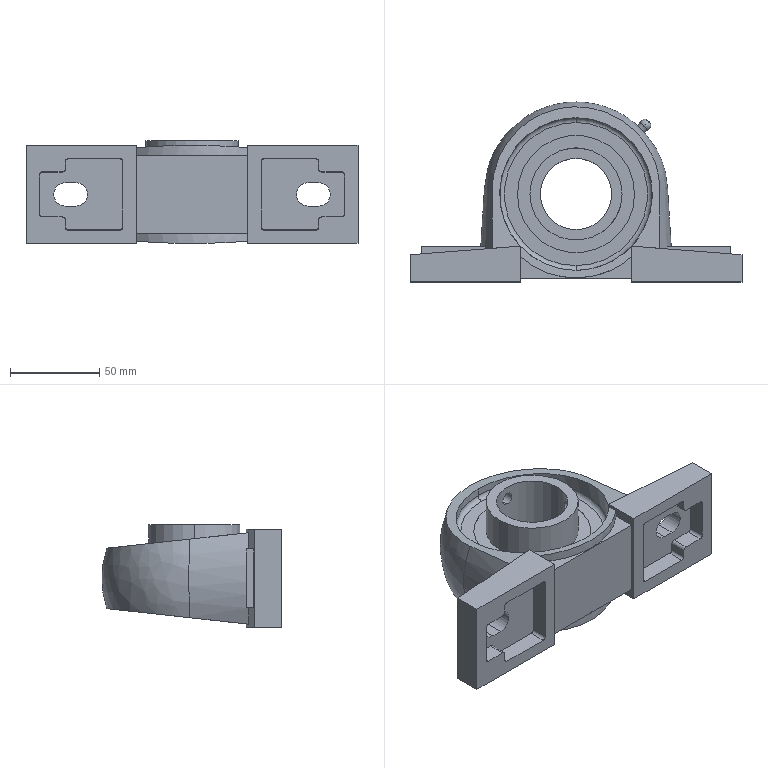Part | SolidWorks | features Revolution 5, Boss 3, Cut 3, CirPattern 2, RevCut 2, Extrusion 1, RefAxis 1, SweepCut 1 | 1 solid | 149 faces | box 186 x 100.8 x 57.7 mm | volume 292850 mm3 | plane 58 | sphere 34 | cylinder 30 | cone 16 | torus 8 | spline 3 | commonest cylinder face diameters 51.6 x6 65.64 x6 85.524 x6 7.134 x4 13 x4 40 x2